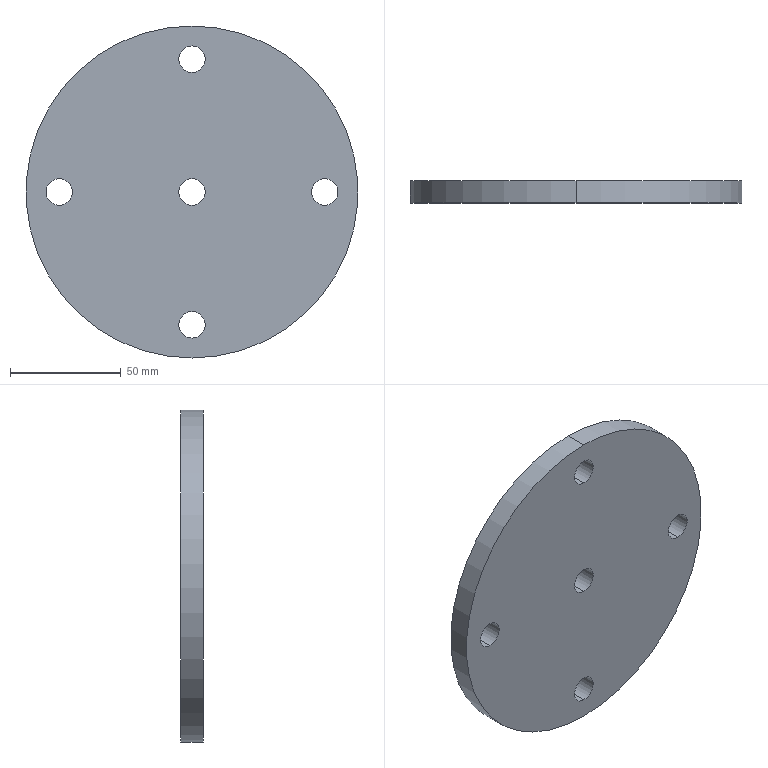Part | SolidWorks | features Extrusion 1, ICE 1 | 1 solid | 14 faces | box 150 x 10 x 150 mm | volume 171060 mm3 | cylinder 12 | plane 2 | commonest cylinder face diameters 12 x10 150 x2
STEP:
#1=CARTESIAN_POINT('',(0.,0.,-66.));
#2=VERTEX_POINT('',#1);
#3=CARTESIAN_POINT('',(0.,0.,-54.));
#4=VERTEX_POINT('',#3);
#5=CARTESIAN_POINT('',(0.,0.,-60.));
#6=DIRECTION('',(0.,1.,0.));
#7=DIRECTION('',(0.,0.,1.));
#8=AXIS2_PLACEMENT_3D('',#5,#6,#7);
#9=CIRCLE('',#8,6.);
#10=EDGE_CURVE('',#2,#4,#9,.T.);
#11=ORIENTED_EDGE('',*,*,#10,.F.);
#12=CARTESIAN_POINT('',(0.,10.,-66.));
#13=VERTEX_POINT('',#12);
#14=CARTESIAN_POINT('',(0.,0.,-66.));
#15=DIRECTION('',(0.,1.,0.));
#16=VECTOR('',#15,1000.);
#17=LINE('',#14,#16);
#18=EDGE_CURVE('',#2,#13,#17,.T.);
#19=ORIENTED_EDGE('',*,*,#18,.T.);
#20=CARTESIAN_POINT('',(0.,10.,-54.));
#21=VERTEX_POINT('',#20);
#22=CARTESIAN_POINT('',(0.,10.,-60.));
#23=DIRECTION('',(0.,1.,0.));
#24=DIRECTION('',(0.,0.,1.));
#25=AXIS2_PLACEMENT_3D('',#22,#23,#24);
#26=CIRCLE('',#25,6.);
#27=EDGE_CURVE('',#13,#21,#26,.T.);
#28=ORIENTED_EDGE('',*,*,#27,.T.);
#29=CARTESIAN_POINT('',(0.,0.,-54.));
#30=DIRECTION('',(0.,1.,0.));
#31=VECTOR('',#30,1000.);
#32=LINE('',#29,#31);
#33=EDGE_CURVE('',#4,#21,#32,.T.);
#34=ORIENTED_EDGE('',*,*,#33,.F.);
#35=EDGE_LOOP('',(#11,#19,#28,#34));
#36=FACE_OUTER_BOUND('',#35,.T.);
#37=CARTESIAN_POINT('',(0.,0.,-60.));
#38=DIRECTION('',(0.,1.,0.));
#39=DIRECTION('',(0.,0.,1.));
#40=AXIS2_PLACEMENT_3D('',#37,#38,#39);
#41=CYLINDRICAL_SURFACE('',#40,6.);
#42=ADVANCED_FACE('',(#36),#41,.F.);
#43=CARTESIAN_POINT('',(60.,0.,-6.));
#44=VERTEX_POINT('',#43);
#45=CARTESIAN_POINT('',(60.,0.,6.));
#46=VERTEX_POINT('',#45);
#47=CARTESIAN_POINT('',(60.,0.,0.));
#48=DIRECTION('',(0.,1.,0.));
#49=DIRECTION('',(0.,0.,1.));
#50=AXIS2_PLACEMENT_3D('',#47,#48,#49);
#51=CIRCLE('',#50,6.);
#52=EDGE_CURVE('',#44,#46,#51,.T.);
#53=ORIENTED_EDGE('',*,*,#52,.F.);
#54=CARTESIAN_POINT('',(60.,10.,-6.));
#55=VERTEX_POINT('',#54);
#56=CARTESIAN_POINT('',(60.,0.,-6.));
#57=DIRECTION('',(0.,1.,0.));
#58=VECTOR('',#57,1000.);
#59=LINE('',#56,#58);
#60=EDGE_CURVE('',#44,#55,#59,.T.);
#61=ORIENTED_EDGE('',*,*,#60,.T.);
#62=CARTESIAN_POINT('',(60.,10.,6.));
#63=VERTEX_POINT('',#62);
#64=CARTESIAN_POINT('',(60.,10.,0.));
#65=DIRECTION('',(0.,1.,0.));
#66=DIRECTION('',(0.,0.,1.));
#67=AXIS2_PLACEMENT_3D('',#64,#65,#66);
#68=CIRCLE('',#67,6.);
#69=EDGE_CURVE('',#55,#63,#68,.T.);
#70=ORIENTED_EDGE('',*,*,#69,.T.);
#71=CARTESIAN_POINT('',(60.,0.,6.));
#72=DIRECTION('',(0.,1.,0.));
#73=VECTOR('',#72,1000.);
#74=LINE('',#71,#73);
#75=EDGE_CURVE('',#46,#63,#74,.T.);
#76=ORIENTED_EDGE('',*,*,#75,.F.);
#77=EDGE_LOOP('',(#53,#61,#70,#76));
#78=FACE_OUTER_BOUND('',#77,.T.);
#79=CARTESIAN_POINT('',(60.,0.,0.));
#80=DIRECTION('',(0.,1.,0.));
#81=DIRECTION('',(0.,0.,1.));
#82=AXIS2_PLACEMENT_3D('',#79,#80,#81);
#83=CYLINDRICAL_SURFACE('',#82,6.);
#84=ADVANCED_FACE('',(#78),#83,.F.);
#85=CARTESIAN_POINT('',(-60.,0.,-6.));
#86=VERTEX_POINT('',#85);
#87=CARTESIAN_POINT('',(-60.,0.,6.));
#88=VERTEX_POINT('',#87);
#89=CARTESIAN_POINT('',(-60.,0.,0.));
#90=DIRECTION('',(0.,1.,0.));
#91=DIRECTION('',(0.,0.,1.));
#92=AXIS2_PLACEMENT_3D('',#89,#90,#91);
#93=CIRCLE('',#92,6.);
#94=EDGE_CURVE('',#86,#88,#93,.T.);
#95=ORIENTED_EDGE('',*,*,#94,.F.);
#96=CARTESIAN_POINT('',(-60.,10.,-6.));
#97=VERTEX_POINT('',#96);
#98=CARTESIAN_POINT('',(-60.,0.,-6.));
#99=DIRECTION('',(0.,1.,0.));
#100=VECTOR('',#99,1000.);
#101=LINE('',#98,#100);
#102=EDGE_CURVE('',#86,#97,#101,.T.);
#103=ORIENTED_EDGE('',*,*,#102,.T.);
#104=CARTESIAN_POINT('',(-60.,10.,6.));
#105=VERTEX_POINT('',#104);
#106=CARTESIAN_POINT('',(-60.,10.,0.));
#107=DIRECTION('',(0.,1.,0.));
#108=DIRECTION('',(0.,0.,1.));
#109=AXIS2_PLACEMENT_3D('',#106,#107,#108);
#110=CIRCLE('',#109,6.);
#111=EDGE_CURVE('',#97,#105,#110,.T.);
#112=ORIENTED_EDGE('',*,*,#111,.T.);
#113=CARTESIAN_POINT('',(-60.,0.,6.));
#114=DIRECTION('',(0.,1.,0.));
#115=VECTOR('',#114,1000.);
#116=LINE('',#113,#115);
#117=EDGE_CURVE('',#88,#105,#116,.T.);
#118=ORIENTED_EDGE('',*,*,#117,.F.);
#119=EDGE_LOOP('',(#95,#103,#112,#118));
#120=FACE_OUTER_BOUND('',#119,.T.);
#121=CARTESIAN_POINT('',(-60.,0.,0.));
#122=DIRECTION('',(0.,1.,0.));
#123=DIRECTION('',(0.,0.,1.));
#124=AXIS2_PLACEMENT_3D('',#121,#122,#123);
#125=CYLINDRICAL_SURFACE('',#124,6.);
#126=ADVANCED_FACE('',(#120),#125,.F.);
#127=CARTESIAN_POINT('',(0.,0.,54.));
#128=VERTEX_POINT('',#127);
#129=CARTESIAN_POINT('',(0.,0.,66.));
#130=VERTEX_POINT('',#129);
#131=CARTESIAN_POINT('',(0.,0.,60.));
#132=DIRECTION('',(0.,1.,0.));
#133=DIRECTION('',(0.,0.,1.));
#134=AXIS2_PLACEMENT_3D('',#131,#132,#133);
#135=CIRCLE('',#134,6.);
#136=EDGE_CURVE('',#128,#130,#135,.T.);
#137=ORIENTED_EDGE('',*,*,#136,.F.);
#138=CARTESIAN_POINT('',(0.,10.,54.));
#139=VERTEX_POINT('',#138);
#140=CARTESIAN_POINT('',(0.,0.,54.));
#141=DIRECTION('',(0.,1.,0.));
#142=VECTOR('',#141,1000.);
#143=LINE('',#140,#142);
#144=EDGE_CURVE('',#128,#139,#143,.T.);
#145=ORIENTED_EDGE('',*,*,#144,.T.);
#146=CARTESIAN_POINT('',(0.,10.,66.));
#147=VERTEX_POINT('',#146);
#148=CARTESIAN_POINT('',(0.,10.,60.));
#149=DIRECTION('',(0.,1.,0.));
#150=DIRECTION('',(0.,0.,1.));
#151=AXIS2_PLACEMENT_3D('',#148,#149,#150);
#152=CIRCLE('',#151,6.);
#153=EDGE_CURVE('',#139,#147,#152,.T.);
#154=ORIENTED_EDGE('',*,*,#153,.T.);
#155=CARTESIAN_POINT('',(0.,0.,66.));
#156=DIRECTION('',(0.,1.,0.));
#157=VECTOR('',#156,1000.);
#158=LINE('',#155,#157);
#159=EDGE_CURVE('',#130,#147,#158,.T.);
#160=ORIENTED_EDGE('',*,*,#159,.F.);
#161=EDGE_LOOP('',(#137,#145,#154,#160));
#162=FACE_OUTER_BOUND('',#161,.T.);
#163=CARTESIAN_POINT('',(0.,0.,60.));
#164=DIRECTION('',(0.,1.,0.));
#165=DIRECTION('',(0.,0.,1.));
#166=AXIS2_PLACEMENT_3D('',#163,#164,#165);
#167=CYLINDRICAL_SURFACE('',#166,6.);
#168=ADVANCED_FACE('',(#162),#167,.F.);
#169=CARTESIAN_POINT('',(0.,0.,-6.));
#170=VERTEX_POINT('',#169);
#171=CARTESIAN_POINT('',(0.,0.,6.));
#172=VERTEX_POINT('',#171);
#173=CARTESIAN_POINT('',(0.,0.,0.));
#174=DIRECTION('',(0.,1.,0.));
#175=DIRECTION('',(0.,0.,1.));
#176=AXIS2_PLACEMENT_3D('',#173,#174,#175);
#177=CIRCLE('',#176,6.);
#178=EDGE_CURVE('',#170,#172,#177,.T.);
#179=ORIENTED_EDGE('',*,*,#178,.F.);
#180=CARTESIAN_POINT('',(0.,10.,-6.));
#181=VERTEX_POINT('',#180);
#182=CARTESIAN_POINT('',(0.,0.,-6.));
#183=DIRECTION('',(0.,1.,0.));
#184=VECTOR('',#183,1000.);
#185=LINE('',#182,#184);
#186=EDGE_CURVE('',#170,#181,#185,.T.);
#187=ORIENTED_EDGE('',*,*,#186,.T.);
#188=CARTESIAN_POINT('',(0.,10.,6.));
#189=VERTEX_POINT('',#188);
#190=CARTESIAN_POINT('',(0.,10.,0.));
#191=DIRECTION('',(0.,1.,0.));
#192=DIRECTION('',(0.,0.,1.));
#193=AXIS2_PLACEMENT_3D('',#190,#191,#192);
#194=CIRCLE('',#193,6.);
#195=EDGE_CURVE('',#181,#189,#194,.T.);
#196=ORIENTED_EDGE('',*,*,#195,.T.);
#197=CARTESIAN_POINT('',(0.,0.,6.));
#198=DIRECTION('',(0.,1.,0.));
#199=VECTOR('',#198,1000.);
#200=LINE('',#197,#199);
#201=EDGE_CURVE('',#172,#189,#200,.T.);
#202=ORIENTED_EDGE('',*,*,#201,.F.);
#203=EDGE_LOOP('',(#179,#187,#196,#202));
#204=FACE_OUTER_BOUND('',#203,.T.);
#205=CARTESIAN_POINT('',(0.,0.,0.));
#206=DIRECTION('',(0.,1.,0.));
#207=DIRECTION('',(0.,0.,1.));
#208=AXIS2_PLACEMENT_3D('',#205,#206,#207);
#209=CYLINDRICAL_SURFACE('',#208,6.);
#210=ADVANCED_FACE('',(#204),#209,.F.);
#211=CARTESIAN_POINT('',(0.,10.,75.));
#212=VERTEX_POINT('',#211);
#213=CARTESIAN_POINT('',(0.,10.,-75.));
#214=VERTEX_POINT('',#213);
#215=CARTESIAN_POINT('',(0.,10.,0.));
#216=DIRECTION('',(0.,1.,0.));
#217=DIRECTION('',(0.,0.,1.));
#218=AXIS2_PLACEMENT_3D('',#215,#216,#217);
#219=CIRCLE('',#218,75.);
#220=EDGE_CURVE('',#212,#214,#219,.T.);
#221=ORIENTED_EDGE('',*,*,#220,.F.);
#222=CARTESIAN_POINT('',(0.,0.,75.));
#223=VERTEX_POINT('',#222);
#224=CARTESIAN_POINT('',(0.,10.,75.));
#225=DIRECTION('',(0.,-1.,0.));
#226=VECTOR('',#225,1000.);
#227=LINE('',#224,#226);
#228=EDGE_CURVE('',#212,#223,#227,.T.);
#229=ORIENTED_EDGE('',*,*,#228,.T.);
#230=CARTESIAN_POINT('',(0.,0.,-75.));
#231=VERTEX_POINT('',#230);
#232=CARTESIAN_POINT('',(0.,0.,0.));
#233=DIRECTION('',(0.,1.,0.));
#234=DIRECTION('',(0.,0.,1.));
#235=AXIS2_PLACEMENT_3D('',#232,#233,#234);
#236=CIRCLE('',#235,75.);
#237=EDGE_CURVE('',#223,#231,#236,.T.);
#238=ORIENTED_EDGE('',*,*,#237,.T.);
#239=CARTESIAN_POINT('',(0.,10.,-75.));
#240=DIRECTION('',(0.,-1.,0.));
#241=VECTOR('',#240,1000.);
#242=LINE('',#239,#241);
#243=EDGE_CURVE('',#214,#231,#242,.T.);
#244=ORIENTED_EDGE('',*,*,#243,.F.);
#245=EDGE_LOOP('',(#221,#229,#238,#244));
#246=FACE_OUTER_BOUND('',#245,.T.);
#247=CARTESIAN_POINT('',(0.,10.,0.));
#248=DIRECTION('',(0.,-1.,0.));
#249=DIRECTION('',(0.,0.,-1.));
#250=AXIS2_PLACEMENT_3D('',#247,#248,#249);
#251=CYLINDRICAL_SURFACE('',#250,75.);
#252=ADVANCED_FACE('',(#246),#251,.T.);
#253=ORIENTED_EDGE('',*,*,#228,.F.);
#254=CARTESIAN_POINT('',(0.,10.,0.));
#255=DIRECTION('',(0.,1.,0.));
#256=DIRECTION('',(0.,0.,1.));
#257=AXIS2_PLACEMENT_3D('',#254,#255,#256);
#258=CIRCLE('',#257,75.);
#259=EDGE_CURVE('',#214,#212,#258,.T.);
#260=ORIENTED_EDGE('',*,*,#259,.F.);
#261=ORIENTED_EDGE('',*,*,#243,.T.);
#262=CARTESIAN_POINT('',(0.,0.,0.));
#263=DIRECTION('',(0.,1.,0.));
#264=DIRECTION('',(0.,0.,1.));
#265=AXIS2_PLACEMENT_3D('',#262,#263,#264);
#266=CIRCLE('',#265,75.);
#267=EDGE_CURVE('',#231,#223,#266,.T.);
#268=ORIENTED_EDGE('',*,*,#267,.T.);
#269=EDGE_LOOP('',(#253,#260,#261,#268));
#270=FACE_OUTER_BOUND('',#269,.T.);
#271=CARTESIAN_POINT('',(0.,10.,0.));
#272=DIRECTION('',(0.,-1.,0.));
#273=DIRECTION('',(0.,0.,-1.));
#274=AXIS2_PLACEMENT_3D('',#271,#272,#273);
#275=CYLINDRICAL_SURFACE('',#274,75.);
#276=ADVANCED_FACE('',(#270),#275,.T.);
#277=CARTESIAN_POINT('',(0.,10.,-60.));
#278=DIRECTION('',(0.,1.,0.));
#279=DIRECTION('',(0.,0.,1.));
#280=AXIS2_PLACEMENT_3D('',#277,#278,#279);
#281=CIRCLE('',#280,6.);
#282=EDGE_CURVE('',#21,#13,#281,.T.);
#283=ORIENTED_EDGE('',*,*,#282,.F.);
#284=ORIENTED_EDGE('',*,*,#27,.F.);
#285=EDGE_LOOP('',(#283,#284));
#286=FACE_BOUND('',#285,.T.);
#287=CARTESIAN_POINT('',(60.,10.,0.));
#288=DIRECTION('',(0.,1.,0.));
#289=DIRECTION('',(0.,0.,1.));
#290=AXIS2_PLACEMENT_3D('',#287,#288,#289);
#291=CIRCLE('',#290,6.);
#292=EDGE_CURVE('',#63,#55,#291,.T.);
#293=ORIENTED_EDGE('',*,*,#292,.F.);
#294=ORIENTED_EDGE('',*,*,#69,.F.);
#295=EDGE_LOOP('',(#293,#294));
#296=FACE_BOUND('',#295,.T.);
#297=CARTESIAN_POINT('',(-60.,10.,0.));
#298=DIRECTION('',(0.,1.,0.));
#299=DIRECTION('',(0.,0.,1.));
#300=AXIS2_PLACEMENT_3D('',#297,#298,#299);
#301=CIRCLE('',#300,6.);
#302=EDGE_CURVE('',#105,#97,#301,.T.);
#303=ORIENTED_EDGE('',*,*,#302,.F.);
#304=ORIENTED_EDGE('',*,*,#111,.F.);
#305=EDGE_LOOP('',(#303,#304));
#306=FACE_BOUND('',#305,.T.);
#307=CARTESIAN_POINT('',(0.,10.,60.));
#308=DIRECTION('',(0.,1.,0.));
#309=DIRECTION('',(0.,0.,1.));
#310=AXIS2_PLACEMENT_3D('',#307,#308,#309);
#311=CIRCLE('',#310,6.);
#312=EDGE_CURVE('',#147,#139,#311,.T.);
#313=ORIENTED_EDGE('',*,*,#312,.F.);
#314=ORIENTED_EDGE('',*,*,#153,.F.);
#315=EDGE_LOOP('',(#313,#314));
#316=FACE_BOUND('',#315,.T.);
#317=CARTESIAN_POINT('',(0.,10.,0.));
#318=DIRECTION('',(0.,1.,0.));
#319=DIRECTION('',(0.,0.,1.));
#320=AXIS2_PLACEMENT_3D('',#317,#318,#319);
#321=CIRCLE('',#320,6.);
#322=EDGE_CURVE('',#189,#181,#321,.T.);
#323=ORIENTED_EDGE('',*,*,#322,.F.);
#324=ORIENTED_EDGE('',*,*,#195,.F.);
#325=EDGE_LOOP('',(#323,#324));
#326=FACE_BOUND('',#325,.T.);
#327=ORIENTED_EDGE('',*,*,#259,.T.);
#328=ORIENTED_EDGE('',*,*,#220,.T.);
#329=EDGE_LOOP('',(#327,#328));
#330=FACE_OUTER_BOUND('',#329,.T.);
#331=CARTESIAN_POINT('',(0.,10.,0.));
#332=DIRECTION('',(0.,1.,0.));
#333=DIRECTION('',(0.,0.,1.));
#334=AXIS2_PLACEMENT_3D('',#331,#332,#333);
#335=PLANE('',#334);
#336=ADVANCED_FACE('',(#286,#296,#306,#316,#326,#330),#335,.T.);
#337=CARTESIAN_POINT('',(0.,0.,-60.));
#338=DIRECTION('',(0.,1.,0.));
#339=DIRECTION('',(0.,0.,1.));
#340=AXIS2_PLACEMENT_3D('',#337,#338,#339);
#341=CIRCLE('',#340,6.);
#342=EDGE_CURVE('',#4,#2,#341,.T.);
#343=ORIENTED_EDGE('',*,*,#342,.T.);
#344=ORIENTED_EDGE('',*,*,#10,.T.);
#345=EDGE_LOOP('',(#343,#344));
#346=FACE_BOUND('',#345,.T.);
#347=CARTESIAN_POINT('',(60.,0.,0.));
#348=DIRECTION('',(0.,1.,0.));
#349=DIRECTION('',(0.,0.,1.));
#350=AXIS2_PLACEMENT_3D('',#347,#348,#349);
#351=CIRCLE('',#350,6.);
#352=EDGE_CURVE('',#46,#44,#351,.T.);
#353=ORIENTED_EDGE('',*,*,#352,.T.);
#354=ORIENTED_EDGE('',*,*,#52,.T.);
#355=EDGE_LOOP('',(#353,#354));
#356=FACE_BOUND('',#355,.T.);
#357=CARTESIAN_POINT('',(-60.,0.,0.));
#358=DIRECTION('',(0.,1.,0.));
#359=DIRECTION('',(0.,0.,1.));
#360=AXIS2_PLACEMENT_3D('',#357,#358,#359);
#361=CIRCLE('',#360,6.);
#362=EDGE_CURVE('',#88,#86,#361,.T.);
#363=ORIENTED_EDGE('',*,*,#362,.T.);
#364=ORIENTED_EDGE('',*,*,#94,.T.);
#365=EDGE_LOOP('',(#363,#364));
#366=FACE_BOUND('',#365,.T.);
#367=CARTESIAN_POINT('',(0.,0.,60.));
#368=DIRECTION('',(0.,1.,0.));
#369=DIRECTION('',(0.,0.,1.));
#370=AXIS2_PLACEMENT_3D('',#367,#368,#369);
#371=CIRCLE('',#370,6.);
#372=EDGE_CURVE('',#130,#128,#371,.T.);
#373=ORIENTED_EDGE('',*,*,#372,.T.);
#374=ORIENTED_EDGE('',*,*,#136,.T.);
#375=EDGE_LOOP('',(#373,#374));
#376=FACE_BOUND('',#375,.T.);
#377=CARTESIAN_POINT('',(0.,0.,0.));
#378=DIRECTION('',(0.,1.,0.));
#379=DIRECTION('',(0.,0.,1.));
#380=AXIS2_PLACEMENT_3D('',#377,#378,#379);
#381=CIRCLE('',#380,6.);
#382=EDGE_CURVE('',#172,#170,#381,.T.);
#383=ORIENTED_EDGE('',*,*,#382,.T.);
#384=ORIENTED_EDGE('',*,*,#178,.T.);
#385=EDGE_LOOP('',(#383,#384));
#386=FACE_BOUND('',#385,.T.);
#387=ORIENTED_EDGE('',*,*,#267,.F.);
#388=ORIENTED_EDGE('',*,*,#237,.F.);
#389=EDGE_LOOP('',(#387,#388));
#390=FACE_OUTER_BOUND('',#389,.T.);
#391=CARTESIAN_POINT('',(0.,0.,0.));
#392=DIRECTION('',(0.,1.,0.));
#393=DIRECTION('',(0.,0.,1.));
#394=AXIS2_PLACEMENT_3D('',#391,#392,#393);
#395=PLANE('',#394);
#396=ADVANCED_FACE('',(#346,#356,#366,#376,#386,#390),#395,.F.);
#397=ORIENTED_EDGE('',*,*,#186,.F.);
#398=ORIENTED_EDGE('',*,*,#382,.F.);
#399=ORIENTED_EDGE('',*,*,#201,.T.);
#400=ORIENTED_EDGE('',*,*,#322,.T.);
#401=EDGE_LOOP('',(#397,#398,#399,#400));
#402=FACE_OUTER_BOUND('',#401,.T.);
#403=CARTESIAN_POINT('',(0.,0.,0.));
#404=DIRECTION('',(0.,1.,0.));
#405=DIRECTION('',(0.,0.,1.));
#406=AXIS2_PLACEMENT_3D('',#403,#404,#405);
#407=CYLINDRICAL_SURFACE('',#406,6.);
#408=ADVANCED_FACE('',(#402),#407,.F.);
#409=ORIENTED_EDGE('',*,*,#144,.F.);
#410=ORIENTED_EDGE('',*,*,#372,.F.);
#411=ORIENTED_EDGE('',*,*,#159,.T.);
#412=ORIENTED_EDGE('',*,*,#312,.T.);
#413=EDGE_LOOP('',(#409,#410,#411,#412));
#414=FACE_OUTER_BOUND('',#413,.T.);
#415=CARTESIAN_POINT('',(0.,0.,60.));
#416=DIRECTION('',(0.,1.,0.));
#417=DIRECTION('',(0.,0.,1.));
#418=AXIS2_PLACEMENT_3D('',#415,#416,#417);
#419=CYLINDRICAL_SURFACE('',#418,6.);
#420=ADVANCED_FACE('',(#414),#419,.F.);
#421=ORIENTED_EDGE('',*,*,#102,.F.);
#422=ORIENTED_EDGE('',*,*,#362,.F.);
#423=ORIENTED_EDGE('',*,*,#117,.T.);
#424=ORIENTED_EDGE('',*,*,#302,.T.);
#425=EDGE_LOOP('',(#421,#422,#423,#424));
#426=FACE_OUTER_BOUND('',#425,.T.);
#427=CARTESIAN_POINT('',(-60.,0.,0.));
#428=DIRECTION('',(0.,1.,0.));
#429=DIRECTION('',(0.,0.,1.));
#430=AXIS2_PLACEMENT_3D('',#427,#428,#429);
#431=CYLINDRICAL_SURFACE('',#430,6.);
#432=ADVANCED_FACE('',(#426),#431,.F.);
#433=ORIENTED_EDGE('',*,*,#60,.F.);
#434=ORIENTED_EDGE('',*,*,#352,.F.);
#435=ORIENTED_EDGE('',*,*,#75,.T.);
#436=ORIENTED_EDGE('',*,*,#292,.T.);
#437=EDGE_LOOP('',(#433,#434,#435,#436));
#438=FACE_OUTER_BOUND('',#437,.T.);
#439=CARTESIAN_POINT('',(60.,0.,0.));
#440=DIRECTION('',(0.,1.,0.));
#441=DIRECTION('',(0.,0.,1.));
#442=AXIS2_PLACEMENT_3D('',#439,#440,#441);
#443=CYLINDRICAL_SURFACE('',#442,6.);
#444=ADVANCED_FACE('',(#438),#443,.F.);
#445=ORIENTED_EDGE('',*,*,#18,.F.);
#446=ORIENTED_EDGE('',*,*,#342,.F.);
#447=ORIENTED_EDGE('',*,*,#33,.T.);
#448=ORIENTED_EDGE('',*,*,#282,.T.);
#449=EDGE_LOOP('',(#445,#446,#447,#448));
#450=FACE_OUTER_BOUND('',#449,.T.);
#451=CARTESIAN_POINT('',(0.,0.,-60.));
#452=DIRECTION('',(0.,1.,0.));
#453=DIRECTION('',(0.,0.,1.));
#454=AXIS2_PLACEMENT_3D('',#451,#452,#453);
#455=CYLINDRICAL_SURFACE('',#454,6.);
#456=ADVANCED_FACE('',(#450),#455,.F.);
#457=CLOSED_SHELL('',(#42,#84,#126,#168,#210,#252,#276,#336,#396,#408,#420,#432,#444,#456));
#458=MANIFOLD_SOLID_BREP('',#457);
#459=CARTESIAN_POINT('',(0.,0.,0.));
#460=DIRECTION('',(0.,0.,1.));
#461=DIRECTION('',(1.,0.,0.));
#462=AXIS2_PLACEMENT_3D('',#459,#460,#461);
#463=(LENGTH_UNIT()NAMED_UNIT(*)SI_UNIT(.MILLI.,.METRE.));
#464=UNCERTAINTY_MEASURE_WITH_UNIT(LENGTH_MEASURE(0.00001),#463,'','');
#465=(NAMED_UNIT(*)PLANE_ANGLE_UNIT()SI_UNIT($,.RADIAN.));
#466=(NAMED_UNIT(*)SI_UNIT($,.STERADIAN.)SOLID_ANGLE_UNIT());
#467=(GEOMETRIC_REPRESENTATION_CONTEXT(3)GLOBAL_UNCERTAINTY_ASSIGNED_CONTEXT((#464))GLOBAL_UNIT_ASSIGNED_CONTEXT((#463,#465,#466))REPRESENTATION_CONTEXT('',''));
#468=ADVANCED_BREP_SHAPE_REPRESENTATION('',(#458,#462),#467);